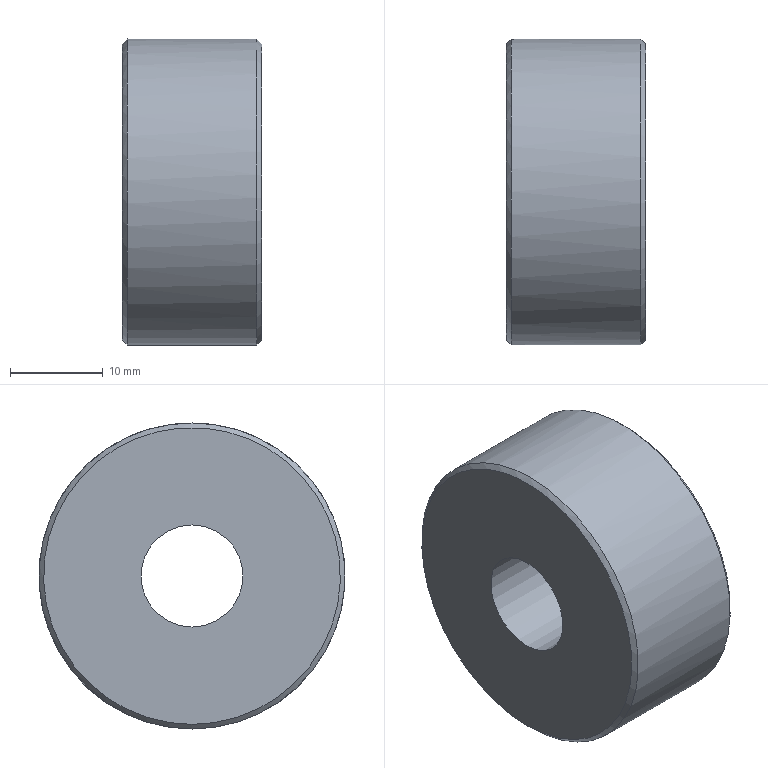Part | STEP file | YBQDJ-FLJ-7 | 1 solid | 6 faces | box 15 x 33 x 33 mm | volume 11378 mm3 | plane 2 | cylinder 2 | cone 2 | commonest cylinder face diameters 11 x1 33 x1
STEP:
#1=CARTESIAN_POINT('',(0.,0.,0.));
#2=DIRECTION('',(0.,0.,1.));
#3=DIRECTION('',(1.,0.,0.));
#4=AXIS2_PLACEMENT_3D('',#1,#2,#3);
#5=CARTESIAN_POINT('',(451.5,-240.,-231.));
#6=VERTEX_POINT('',#5);
#7=CARTESIAN_POINT('',(451.5,-240.,-215.));
#8=DIRECTION('',(-1.,0.,0.));
#9=DIRECTION('',(0.,0.,-1.));
#10=AXIS2_PLACEMENT_3D('',#7,#8,#9);
#11=CIRCLE('',#10,16.);
#12=CARTESIAN_POINT('',(451.5,-240.,-215.));
#13=DIRECTION('',(1.,0.,0.));
#14=DIRECTION('',(0.,0.,-1.));
#15=AXIS2_PLACEMENT_3D('',#12,#13,#14);
#16=PLANE('',#15);
#17=CARTESIAN_POINT('',(16.,0.));
#18=CARTESIAN_POINT('',(16.,-27.713));
#19=CARTESIAN_POINT('',(-8.,-13.856));
#20=CARTESIAN_POINT('',(-32.,0.));
#21=CARTESIAN_POINT('',(-8.,13.856));
#22=CARTESIAN_POINT('',(16.,27.713));
#23=CARTESIAN_POINT('',(16.,0.));
#24=(BOUNDED_CURVE()B_SPLINE_CURVE(2,(#17,#18,#19,#20,#21,#22,#23),.UNSPECIFIED.,.T.,.F.)B_SPLINE_CURVE_WITH_KNOTS((1,2,2,2,2,1),(-2.094,0.,2.094,4.189,6.283,8.378),.UNSPECIFIED.)CURVE()GEOMETRIC_REPRESENTATION_ITEM()RATIONAL_B_SPLINE_CURVE((1.,0.5,1.,0.5,1.,0.5,1.))REPRESENTATION_ITEM(''));
#25=(GEOMETRIC_REPRESENTATION_CONTEXT(2)PARAMETRIC_REPRESENTATION_CONTEXT()REPRESENTATION_CONTEXT('',''));
#26=DEFINITIONAL_REPRESENTATION('',(#24),#25);
#27=PCURVE('',#16,#26);
#28=CARTESIAN_POINT('',(451.5,-240.,-215.));
#29=DIRECTION('',(1.,0.,0.));
#30=DIRECTION('',(0.,0.,-1.));
#31=AXIS2_PLACEMENT_3D('',#28,#29,#30);
#32=CONICAL_SURFACE('',#31,16.,0.7854);
#33=CARTESIAN_POINT('',(6.283,0.));
#34=DIRECTION('',(-1.,0.));
#35=VECTOR('',#34,1.);
#36=LINE('',#33,#35);
#37=(GEOMETRIC_REPRESENTATION_CONTEXT(2)PARAMETRIC_REPRESENTATION_CONTEXT()REPRESENTATION_CONTEXT('',''));
#38=DEFINITIONAL_REPRESENTATION('',(#36),#37);
#39=PCURVE('',#32,#38);
#40=SURFACE_CURVE('',#11,(#27,#39),.PCURVE_S1.);
#41=EDGE_CURVE('',#6,#6,#40,.T.);
#42=ORIENTED_EDGE('',*,*,#41,.T.);
#43=EDGE_LOOP('',(#42));
#44=FACE_BOUND('',#43,.T.);
#45=CARTESIAN_POINT('',(451.5,-240.,-220.5));
#46=VERTEX_POINT('',#45);
#47=CARTESIAN_POINT('',(451.5,-240.,-215.));
#48=DIRECTION('',(-1.,0.,0.));
#49=DIRECTION('',(0.,0.,-1.));
#50=AXIS2_PLACEMENT_3D('',#47,#48,#49);
#51=CIRCLE('',#50,5.5);
#52=CARTESIAN_POINT('',(5.5,0.));
#53=CARTESIAN_POINT('',(5.5,-9.526));
#54=CARTESIAN_POINT('',(-2.75,-4.763));
#55=CARTESIAN_POINT('',(-11.,0.));
#56=CARTESIAN_POINT('',(-2.75,4.763));
#57=CARTESIAN_POINT('',(5.5,9.526));
#58=CARTESIAN_POINT('',(5.5,0.));
#59=(BOUNDED_CURVE()B_SPLINE_CURVE(2,(#52,#53,#54,#55,#56,#57,#58),.UNSPECIFIED.,.T.,.F.)B_SPLINE_CURVE_WITH_KNOTS((1,2,2,2,2,1),(-2.094,0.,2.094,4.189,6.283,8.378),.UNSPECIFIED.)CURVE()GEOMETRIC_REPRESENTATION_ITEM()RATIONAL_B_SPLINE_CURVE((1.,0.5,1.,0.5,1.,0.5,1.))REPRESENTATION_ITEM(''));
#60=(GEOMETRIC_REPRESENTATION_CONTEXT(2)PARAMETRIC_REPRESENTATION_CONTEXT()REPRESENTATION_CONTEXT('',''));
#61=DEFINITIONAL_REPRESENTATION('',(#59),#60);
#62=PCURVE('',#16,#61);
#63=CARTESIAN_POINT('',(451.5,-240.,-215.));
#64=DIRECTION('',(1.,0.,0.));
#65=DIRECTION('',(0.,0.,-1.));
#66=AXIS2_PLACEMENT_3D('',#63,#64,#65);
#67=CYLINDRICAL_SURFACE('',#66,5.5);
#68=CARTESIAN_POINT('',(6.283,0.));
#69=DIRECTION('',(-1.,0.));
#70=VECTOR('',#69,1.);
#71=LINE('',#68,#70);
#72=(GEOMETRIC_REPRESENTATION_CONTEXT(2)PARAMETRIC_REPRESENTATION_CONTEXT()REPRESENTATION_CONTEXT('',''));
#73=DEFINITIONAL_REPRESENTATION('',(#71),#72);
#74=PCURVE('',#67,#73);
#75=SURFACE_CURVE('',#51,(#62,#74),.PCURVE_S1.);
#76=EDGE_CURVE('',#46,#46,#75,.T.);
#77=ORIENTED_EDGE('',*,*,#76,.F.);
#78=EDGE_LOOP('',(#77));
#79=FACE_BOUND('',#78,.T.);
#80=ADVANCED_FACE('',(#44,#79),#16,.F.);
#81=CARTESIAN_POINT('',(466.5,-240.,-231.));
#82=VERTEX_POINT('',#81);
#83=CARTESIAN_POINT('',(466.5,-240.,-215.));
#84=DIRECTION('',(1.,0.,0.));
#85=DIRECTION('',(0.,0.,-1.));
#86=AXIS2_PLACEMENT_3D('',#83,#84,#85);
#87=CIRCLE('',#86,16.);
#88=CARTESIAN_POINT('',(466.5,-240.,-215.));
#89=DIRECTION('',(1.,0.,0.));
#90=DIRECTION('',(0.,0.,-1.));
#91=AXIS2_PLACEMENT_3D('',#88,#89,#90);
#92=PLANE('',#91);
#93=CARTESIAN_POINT('',(0.,0.));
#94=DIRECTION('',(1.,0.));
#95=AXIS2_PLACEMENT_2D('',#93,#94);
#96=CIRCLE('',#95,16.);
#97=(GEOMETRIC_REPRESENTATION_CONTEXT(2)PARAMETRIC_REPRESENTATION_CONTEXT()REPRESENTATION_CONTEXT('',''));
#98=DEFINITIONAL_REPRESENTATION('',(#96),#97);
#99=PCURVE('',#92,#98);
#100=CARTESIAN_POINT('',(466.,-240.,-215.));
#101=DIRECTION('',(-1.,0.,0.));
#102=DIRECTION('',(0.,0.,1.));
#103=AXIS2_PLACEMENT_3D('',#100,#101,#102);
#104=CONICAL_SURFACE('',#103,16.5,0.7854);
#105=CARTESIAN_POINT('',(9.425,-0.5));
#106=DIRECTION('',(-1.,0.));
#107=VECTOR('',#106,1.);
#108=LINE('',#105,#107);
#109=(GEOMETRIC_REPRESENTATION_CONTEXT(2)PARAMETRIC_REPRESENTATION_CONTEXT()REPRESENTATION_CONTEXT('',''));
#110=DEFINITIONAL_REPRESENTATION('',(#108),#109);
#111=PCURVE('',#104,#110);
#112=SURFACE_CURVE('',#87,(#99,#111),.PCURVE_S1.);
#113=EDGE_CURVE('',#82,#82,#112,.T.);
#114=ORIENTED_EDGE('',*,*,#113,.T.);
#115=EDGE_LOOP('',(#114));
#116=FACE_BOUND('',#115,.T.);
#117=CARTESIAN_POINT('',(466.5,-240.,-220.5));
#118=VERTEX_POINT('',#117);
#119=CARTESIAN_POINT('',(466.5,-240.,-215.));
#120=DIRECTION('',(-1.,0.,0.));
#121=DIRECTION('',(0.,0.,-1.));
#122=AXIS2_PLACEMENT_3D('',#119,#120,#121);
#123=CIRCLE('',#122,5.5);
#124=CARTESIAN_POINT('',(5.5,0.));
#125=CARTESIAN_POINT('',(5.5,-9.526));
#126=CARTESIAN_POINT('',(-2.75,-4.763));
#127=CARTESIAN_POINT('',(-11.,0.));
#128=CARTESIAN_POINT('',(-2.75,4.763));
#129=CARTESIAN_POINT('',(5.5,9.526));
#130=CARTESIAN_POINT('',(5.5,0.));
#131=(BOUNDED_CURVE()B_SPLINE_CURVE(2,(#124,#125,#126,#127,#128,#129,#130),.UNSPECIFIED.,.T.,.F.)B_SPLINE_CURVE_WITH_KNOTS((1,2,2,2,2,1),(-2.094,0.,2.094,4.189,6.283,8.378),.UNSPECIFIED.)CURVE()GEOMETRIC_REPRESENTATION_ITEM()RATIONAL_B_SPLINE_CURVE((1.,0.5,1.,0.5,1.,0.5,1.))REPRESENTATION_ITEM(''));
#132=(GEOMETRIC_REPRESENTATION_CONTEXT(2)PARAMETRIC_REPRESENTATION_CONTEXT()REPRESENTATION_CONTEXT('',''));
#133=DEFINITIONAL_REPRESENTATION('',(#131),#132);
#134=PCURVE('',#92,#133);
#135=CARTESIAN_POINT('',(6.283,15.));
#136=DIRECTION('',(-1.,0.));
#137=VECTOR('',#136,1.);
#138=LINE('',#135,#137);
#139=(GEOMETRIC_REPRESENTATION_CONTEXT(2)PARAMETRIC_REPRESENTATION_CONTEXT()REPRESENTATION_CONTEXT('',''));
#140=DEFINITIONAL_REPRESENTATION('',(#138),#139);
#141=PCURVE('',#67,#140);
#142=SURFACE_CURVE('',#123,(#134,#141),.PCURVE_S1.);
#143=EDGE_CURVE('',#118,#118,#142,.T.);
#144=ORIENTED_EDGE('',*,*,#143,.T.);
#145=EDGE_LOOP('',(#144));
#146=FACE_BOUND('',#145,.T.);
#147=ADVANCED_FACE('',(#116,#146),#92,.T.);
#148=CARTESIAN_POINT('',(466.,-240.,-231.5));
#149=VERTEX_POINT('',#148);
#150=CARTESIAN_POINT('',(466.,-240.,-215.));
#151=DIRECTION('',(-1.,0.,0.));
#152=DIRECTION('',(0.,0.,-1.));
#153=AXIS2_PLACEMENT_3D('',#150,#151,#152);
#154=CIRCLE('',#153,16.5);
#155=CARTESIAN_POINT('',(451.5,-240.,-215.));
#156=DIRECTION('',(1.,0.,0.));
#157=DIRECTION('',(0.,0.,-1.));
#158=AXIS2_PLACEMENT_3D('',#155,#156,#157);
#159=CYLINDRICAL_SURFACE('',#158,16.5);
#160=CARTESIAN_POINT('',(6.283,14.5));
#161=DIRECTION('',(-1.,0.));
#162=VECTOR('',#161,1.);
#163=LINE('',#160,#162);
#164=(GEOMETRIC_REPRESENTATION_CONTEXT(2)PARAMETRIC_REPRESENTATION_CONTEXT()REPRESENTATION_CONTEXT('',''));
#165=DEFINITIONAL_REPRESENTATION('',(#163),#164);
#166=PCURVE('',#159,#165);
#167=CARTESIAN_POINT('',(3.142,0.));
#168=DIRECTION('',(1.,0.));
#169=VECTOR('',#168,1.);
#170=LINE('',#167,#169);
#171=(GEOMETRIC_REPRESENTATION_CONTEXT(2)PARAMETRIC_REPRESENTATION_CONTEXT()REPRESENTATION_CONTEXT('',''));
#172=DEFINITIONAL_REPRESENTATION('',(#170),#171);
#173=PCURVE('',#104,#172);
#174=SURFACE_CURVE('',#154,(#166,#173),.PCURVE_S1.);
#175=EDGE_CURVE('',#149,#149,#174,.T.);
#176=ORIENTED_EDGE('',*,*,#175,.T.);
#177=CARTESIAN_POINT('',(452.,-240.,-231.5));
#178=VERTEX_POINT('',#177);
#179=CARTESIAN_POINT('',(452.,-240.,-231.5));
#180=CARTESIAN_POINT('',(466.,-240.,-231.5));
#181=B_SPLINE_CURVE_WITH_KNOTS('',1,(#179,#180),.UNSPECIFIED.,.F.,.F.,(2,2),(0.5,14.5),.PIECEWISE_BEZIER_KNOTS.);
#182=CARTESIAN_POINT('',(0.,0.));
#183=DIRECTION('',(0.,1.));
#184=VECTOR('',#183,1.);
#185=LINE('',#182,#184);
#186=(GEOMETRIC_REPRESENTATION_CONTEXT(2)PARAMETRIC_REPRESENTATION_CONTEXT()REPRESENTATION_CONTEXT('',''));
#187=DEFINITIONAL_REPRESENTATION('',(#185),#186);
#188=PCURVE('',#159,#187);
#189=CARTESIAN_POINT('',(6.283,0.));
#190=DIRECTION('',(0.,1.));
#191=VECTOR('',#190,1.);
#192=LINE('',#189,#191);
#193=(GEOMETRIC_REPRESENTATION_CONTEXT(2)PARAMETRIC_REPRESENTATION_CONTEXT()REPRESENTATION_CONTEXT('',''));
#194=DEFINITIONAL_REPRESENTATION('',(#192),#193);
#195=PCURVE('',#159,#194);
#196=SEAM_CURVE('',#181,(#188,#195),.PCURVE_S1.);
#197=EDGE_CURVE('',#178,#149,#196,.T.);
#198=ORIENTED_EDGE('',*,*,#197,.F.);
#199=CARTESIAN_POINT('',(452.,-240.,-198.5));
#200=VERTEX_POINT('',#199);
#201=CARTESIAN_POINT('',(452.,-240.,-215.));
#202=DIRECTION('',(1.,0.,0.));
#203=DIRECTION('',(0.,0.,1.));
#204=AXIS2_PLACEMENT_3D('',#201,#202,#203);
#205=CIRCLE('',#204,16.5);
#206=CARTESIAN_POINT('',(-3.142,0.5));
#207=DIRECTION('',(1.,0.));
#208=VECTOR('',#207,1.);
#209=LINE('',#206,#208);
#210=(GEOMETRIC_REPRESENTATION_CONTEXT(2)PARAMETRIC_REPRESENTATION_CONTEXT()REPRESENTATION_CONTEXT('',''));
#211=DEFINITIONAL_REPRESENTATION('',(#209),#210);
#212=PCURVE('',#159,#211);
#213=CARTESIAN_POINT('',(-3.142,0.5));
#214=DIRECTION('',(1.,0.));
#215=VECTOR('',#214,1.);
#216=LINE('',#213,#215);
#217=(GEOMETRIC_REPRESENTATION_CONTEXT(2)PARAMETRIC_REPRESENTATION_CONTEXT()REPRESENTATION_CONTEXT('',''));
#218=DEFINITIONAL_REPRESENTATION('',(#216),#217);
#219=PCURVE('',#32,#218);
#220=SURFACE_CURVE('',#205,(#212,#219),.PCURVE_S1.);
#221=EDGE_CURVE('',#178,#200,#220,.T.);
#222=ORIENTED_EDGE('',*,*,#221,.T.);
#223=CARTESIAN_POINT('',(452.,-240.,-215.));
#224=DIRECTION('',(1.,0.,0.));
#225=DIRECTION('',(0.,0.,1.));
#226=AXIS2_PLACEMENT_3D('',#223,#224,#225);
#227=CIRCLE('',#226,16.5);
#228=CARTESIAN_POINT('',(3.142,0.5));
#229=DIRECTION('',(1.,0.));
#230=VECTOR('',#229,1.);
#231=LINE('',#228,#230);
#232=(GEOMETRIC_REPRESENTATION_CONTEXT(2)PARAMETRIC_REPRESENTATION_CONTEXT()REPRESENTATION_CONTEXT('',''));
#233=DEFINITIONAL_REPRESENTATION('',(#231),#232);
#234=PCURVE('',#159,#233);
#235=CARTESIAN_POINT('',(3.142,0.5));
#236=DIRECTION('',(1.,0.));
#237=VECTOR('',#236,1.);
#238=LINE('',#235,#237);
#239=(GEOMETRIC_REPRESENTATION_CONTEXT(2)PARAMETRIC_REPRESENTATION_CONTEXT()REPRESENTATION_CONTEXT('',''));
#240=DEFINITIONAL_REPRESENTATION('',(#238),#239);
#241=PCURVE('',#32,#240);
#242=SURFACE_CURVE('',#227,(#234,#241),.PCURVE_S1.);
#243=EDGE_CURVE('',#200,#178,#242,.T.);
#244=ORIENTED_EDGE('',*,*,#243,.T.);
#245=ORIENTED_EDGE('',*,*,#197,.T.);
#246=EDGE_LOOP('',(#176,#198,#222,#244,#245));
#247=FACE_BOUND('',#246,.T.);
#248=ADVANCED_FACE('',(#247),#159,.T.);
#249=ORIENTED_EDGE('',*,*,#76,.F.);
#250=CARTESIAN_POINT('',(451.5,-240.,-220.5));
#251=CARTESIAN_POINT('',(466.5,-240.,-220.5));
#252=B_SPLINE_CURVE_WITH_KNOTS('',1,(#250,#251),.UNSPECIFIED.,.F.,.F.,(2,2),(0.,15.),.PIECEWISE_BEZIER_KNOTS.);
#253=CARTESIAN_POINT('',(6.283,0.));
#254=DIRECTION('',(0.,1.));
#255=VECTOR('',#254,1.);
#256=LINE('',#253,#255);
#257=(GEOMETRIC_REPRESENTATION_CONTEXT(2)PARAMETRIC_REPRESENTATION_CONTEXT()REPRESENTATION_CONTEXT('',''));
#258=DEFINITIONAL_REPRESENTATION('',(#256),#257);
#259=PCURVE('',#67,#258);
#260=CARTESIAN_POINT('',(0.,0.));
#261=DIRECTION('',(0.,1.));
#262=VECTOR('',#261,1.);
#263=LINE('',#260,#262);
#264=(GEOMETRIC_REPRESENTATION_CONTEXT(2)PARAMETRIC_REPRESENTATION_CONTEXT()REPRESENTATION_CONTEXT('',''));
#265=DEFINITIONAL_REPRESENTATION('',(#263),#264);
#266=PCURVE('',#67,#265);
#267=SEAM_CURVE('',#252,(#259,#266),.PCURVE_S1.);
#268=EDGE_CURVE('',#46,#118,#267,.T.);
#269=ORIENTED_EDGE('',*,*,#268,.T.);
#270=ORIENTED_EDGE('',*,*,#143,.T.);
#271=ORIENTED_EDGE('',*,*,#268,.F.);
#272=EDGE_LOOP('',(#249,#269,#270,#271));
#273=FACE_BOUND('',#272,.F.);
#274=ADVANCED_FACE('',(#273),#67,.F.);
#275=ORIENTED_EDGE('',*,*,#113,.F.);
#276=CARTESIAN_POINT('',(466.5,-240.,-231.));
#277=CARTESIAN_POINT('',(466.,-240.,-231.5));
#278=B_SPLINE_CURVE_WITH_KNOTS('',1,(#276,#277),.UNSPECIFIED.,.F.,.F.,(2,2),(-0.7071,0.),.PIECEWISE_BEZIER_KNOTS.);
#279=CARTESIAN_POINT('',(9.425,0.));
#280=DIRECTION('',(0.,1.));
#281=VECTOR('',#280,1.);
#282=LINE('',#279,#281);
#283=(GEOMETRIC_REPRESENTATION_CONTEXT(2)PARAMETRIC_REPRESENTATION_CONTEXT()REPRESENTATION_CONTEXT('',''));
#284=DEFINITIONAL_REPRESENTATION('',(#282),#283);
#285=PCURVE('',#104,#284);
#286=CARTESIAN_POINT('',(3.142,0.));
#287=DIRECTION('',(0.,1.));
#288=VECTOR('',#287,1.);
#289=LINE('',#286,#288);
#290=(GEOMETRIC_REPRESENTATION_CONTEXT(2)PARAMETRIC_REPRESENTATION_CONTEXT()REPRESENTATION_CONTEXT('',''));
#291=DEFINITIONAL_REPRESENTATION('',(#289),#290);
#292=PCURVE('',#104,#291);
#293=SEAM_CURVE('',#278,(#285,#292),.PCURVE_S1.);
#294=EDGE_CURVE('',#82,#149,#293,.T.);
#295=ORIENTED_EDGE('',*,*,#294,.T.);
#296=ORIENTED_EDGE('',*,*,#175,.F.);
#297=ORIENTED_EDGE('',*,*,#294,.F.);
#298=EDGE_LOOP('',(#275,#295,#296,#297));
#299=FACE_BOUND('',#298,.T.);
#300=ADVANCED_FACE('',(#299),#104,.T.);
#301=ORIENTED_EDGE('',*,*,#243,.F.);
#302=ORIENTED_EDGE('',*,*,#221,.F.);
#303=CARTESIAN_POINT('',(451.5,-240.,-231.));
#304=CARTESIAN_POINT('',(452.,-240.,-231.5));
#305=B_SPLINE_CURVE_WITH_KNOTS('',1,(#303,#304),.UNSPECIFIED.,.F.,.F.,(2,2),(0.,0.7071),.PIECEWISE_BEZIER_KNOTS.);
#306=CARTESIAN_POINT('',(0.,0.));
#307=DIRECTION('',(0.,1.));
#308=VECTOR('',#307,1.);
#309=LINE('',#306,#308);
#310=(GEOMETRIC_REPRESENTATION_CONTEXT(2)PARAMETRIC_REPRESENTATION_CONTEXT()REPRESENTATION_CONTEXT('',''));
#311=DEFINITIONAL_REPRESENTATION('',(#309),#310);
#312=PCURVE('',#32,#311);
#313=CARTESIAN_POINT('',(6.283,0.));
#314=DIRECTION('',(0.,1.));
#315=VECTOR('',#314,1.);
#316=LINE('',#313,#315);
#317=(GEOMETRIC_REPRESENTATION_CONTEXT(2)PARAMETRIC_REPRESENTATION_CONTEXT()REPRESENTATION_CONTEXT('',''));
#318=DEFINITIONAL_REPRESENTATION('',(#316),#317);
#319=PCURVE('',#32,#318);
#320=SEAM_CURVE('',#305,(#312,#319),.PCURVE_S1.);
#321=EDGE_CURVE('',#6,#178,#320,.T.);
#322=ORIENTED_EDGE('',*,*,#321,.F.);
#323=ORIENTED_EDGE('',*,*,#41,.F.);
#324=ORIENTED_EDGE('',*,*,#321,.T.);
#325=EDGE_LOOP('',(#301,#302,#322,#323,#324));
#326=FACE_BOUND('',#325,.T.);
#327=ADVANCED_FACE('',(#326),#32,.T.);
#328=CLOSED_SHELL('',(#80,#147,#248,#274,#300,#327));
#329=MANIFOLD_SOLID_BREP('',#328);
#330=(LENGTH_UNIT()NAMED_UNIT(*)SI_UNIT(.MILLI.,.METRE.));
#331=UNCERTAINTY_MEASURE_WITH_UNIT(LENGTH_MEASURE(0.00001),#330,'','');
#332=(NAMED_UNIT(*)PLANE_ANGLE_UNIT()SI_UNIT($,.RADIAN.));
#333=(NAMED_UNIT(*)SI_UNIT($,.STERADIAN.)SOLID_ANGLE_UNIT());
#334=(GEOMETRIC_REPRESENTATION_CONTEXT(3)GLOBAL_UNCERTAINTY_ASSIGNED_CONTEXT((#331))GLOBAL_UNIT_ASSIGNED_CONTEXT((#330,#332,#333))REPRESENTATION_CONTEXT('',''));
#335=ADVANCED_BREP_SHAPE_REPRESENTATION('',(#4,#329),#334);